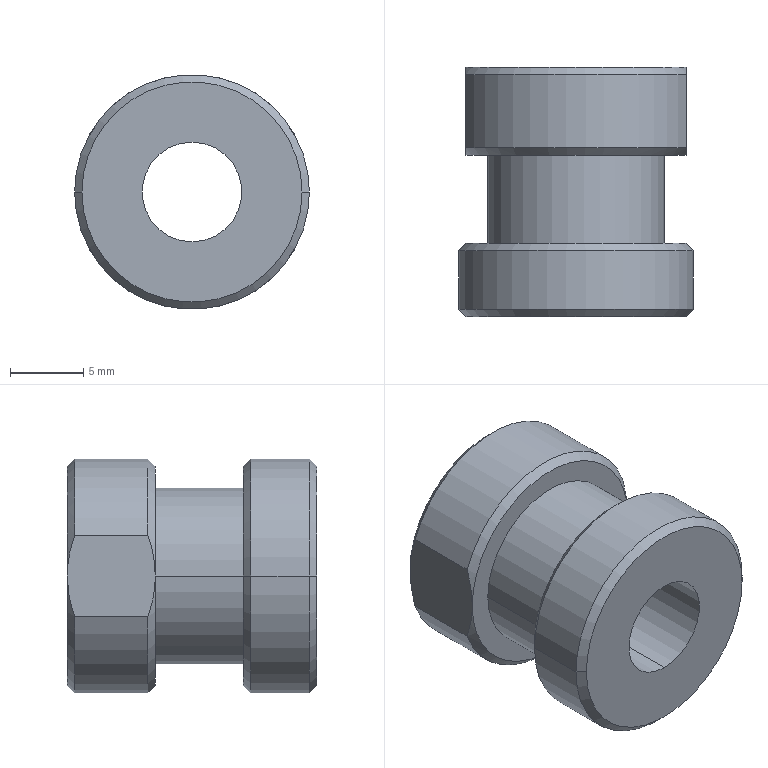Part | STEP file | union | 1 solid | 22 faces | box 16 x 17 x 16 mm | volume 2228 mm3 | cylinder 8 | cone 8 | plane 6 | commonest cylinder face diameters 16 x4 6.8 x2 12 x2